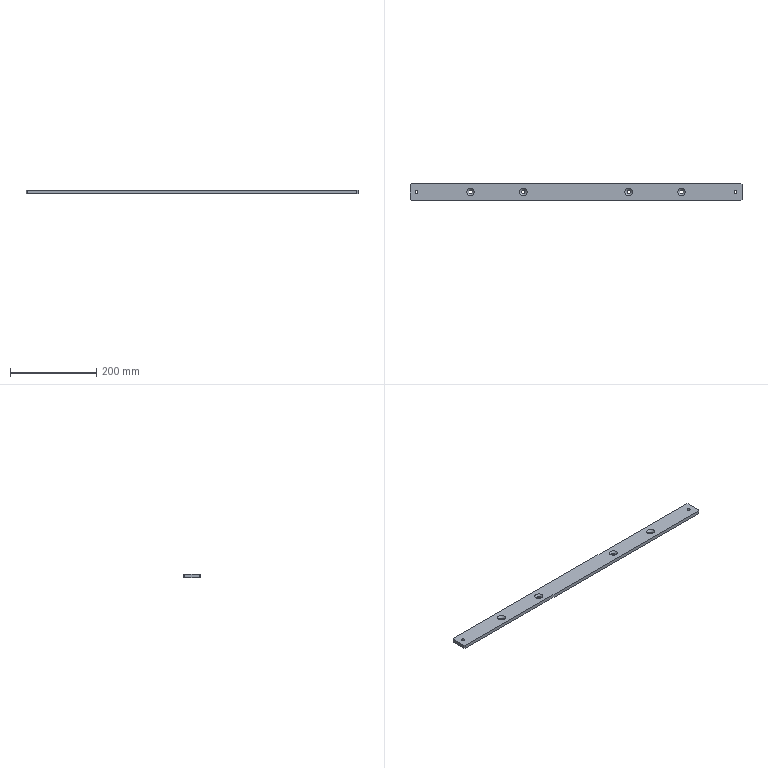Part | STEP file | rectangular profile 40x8 | 1 solid | 20 faces | box 767.8 x 40 x 8 mm | volume 241435 mm3 | spline 10 | plane 10